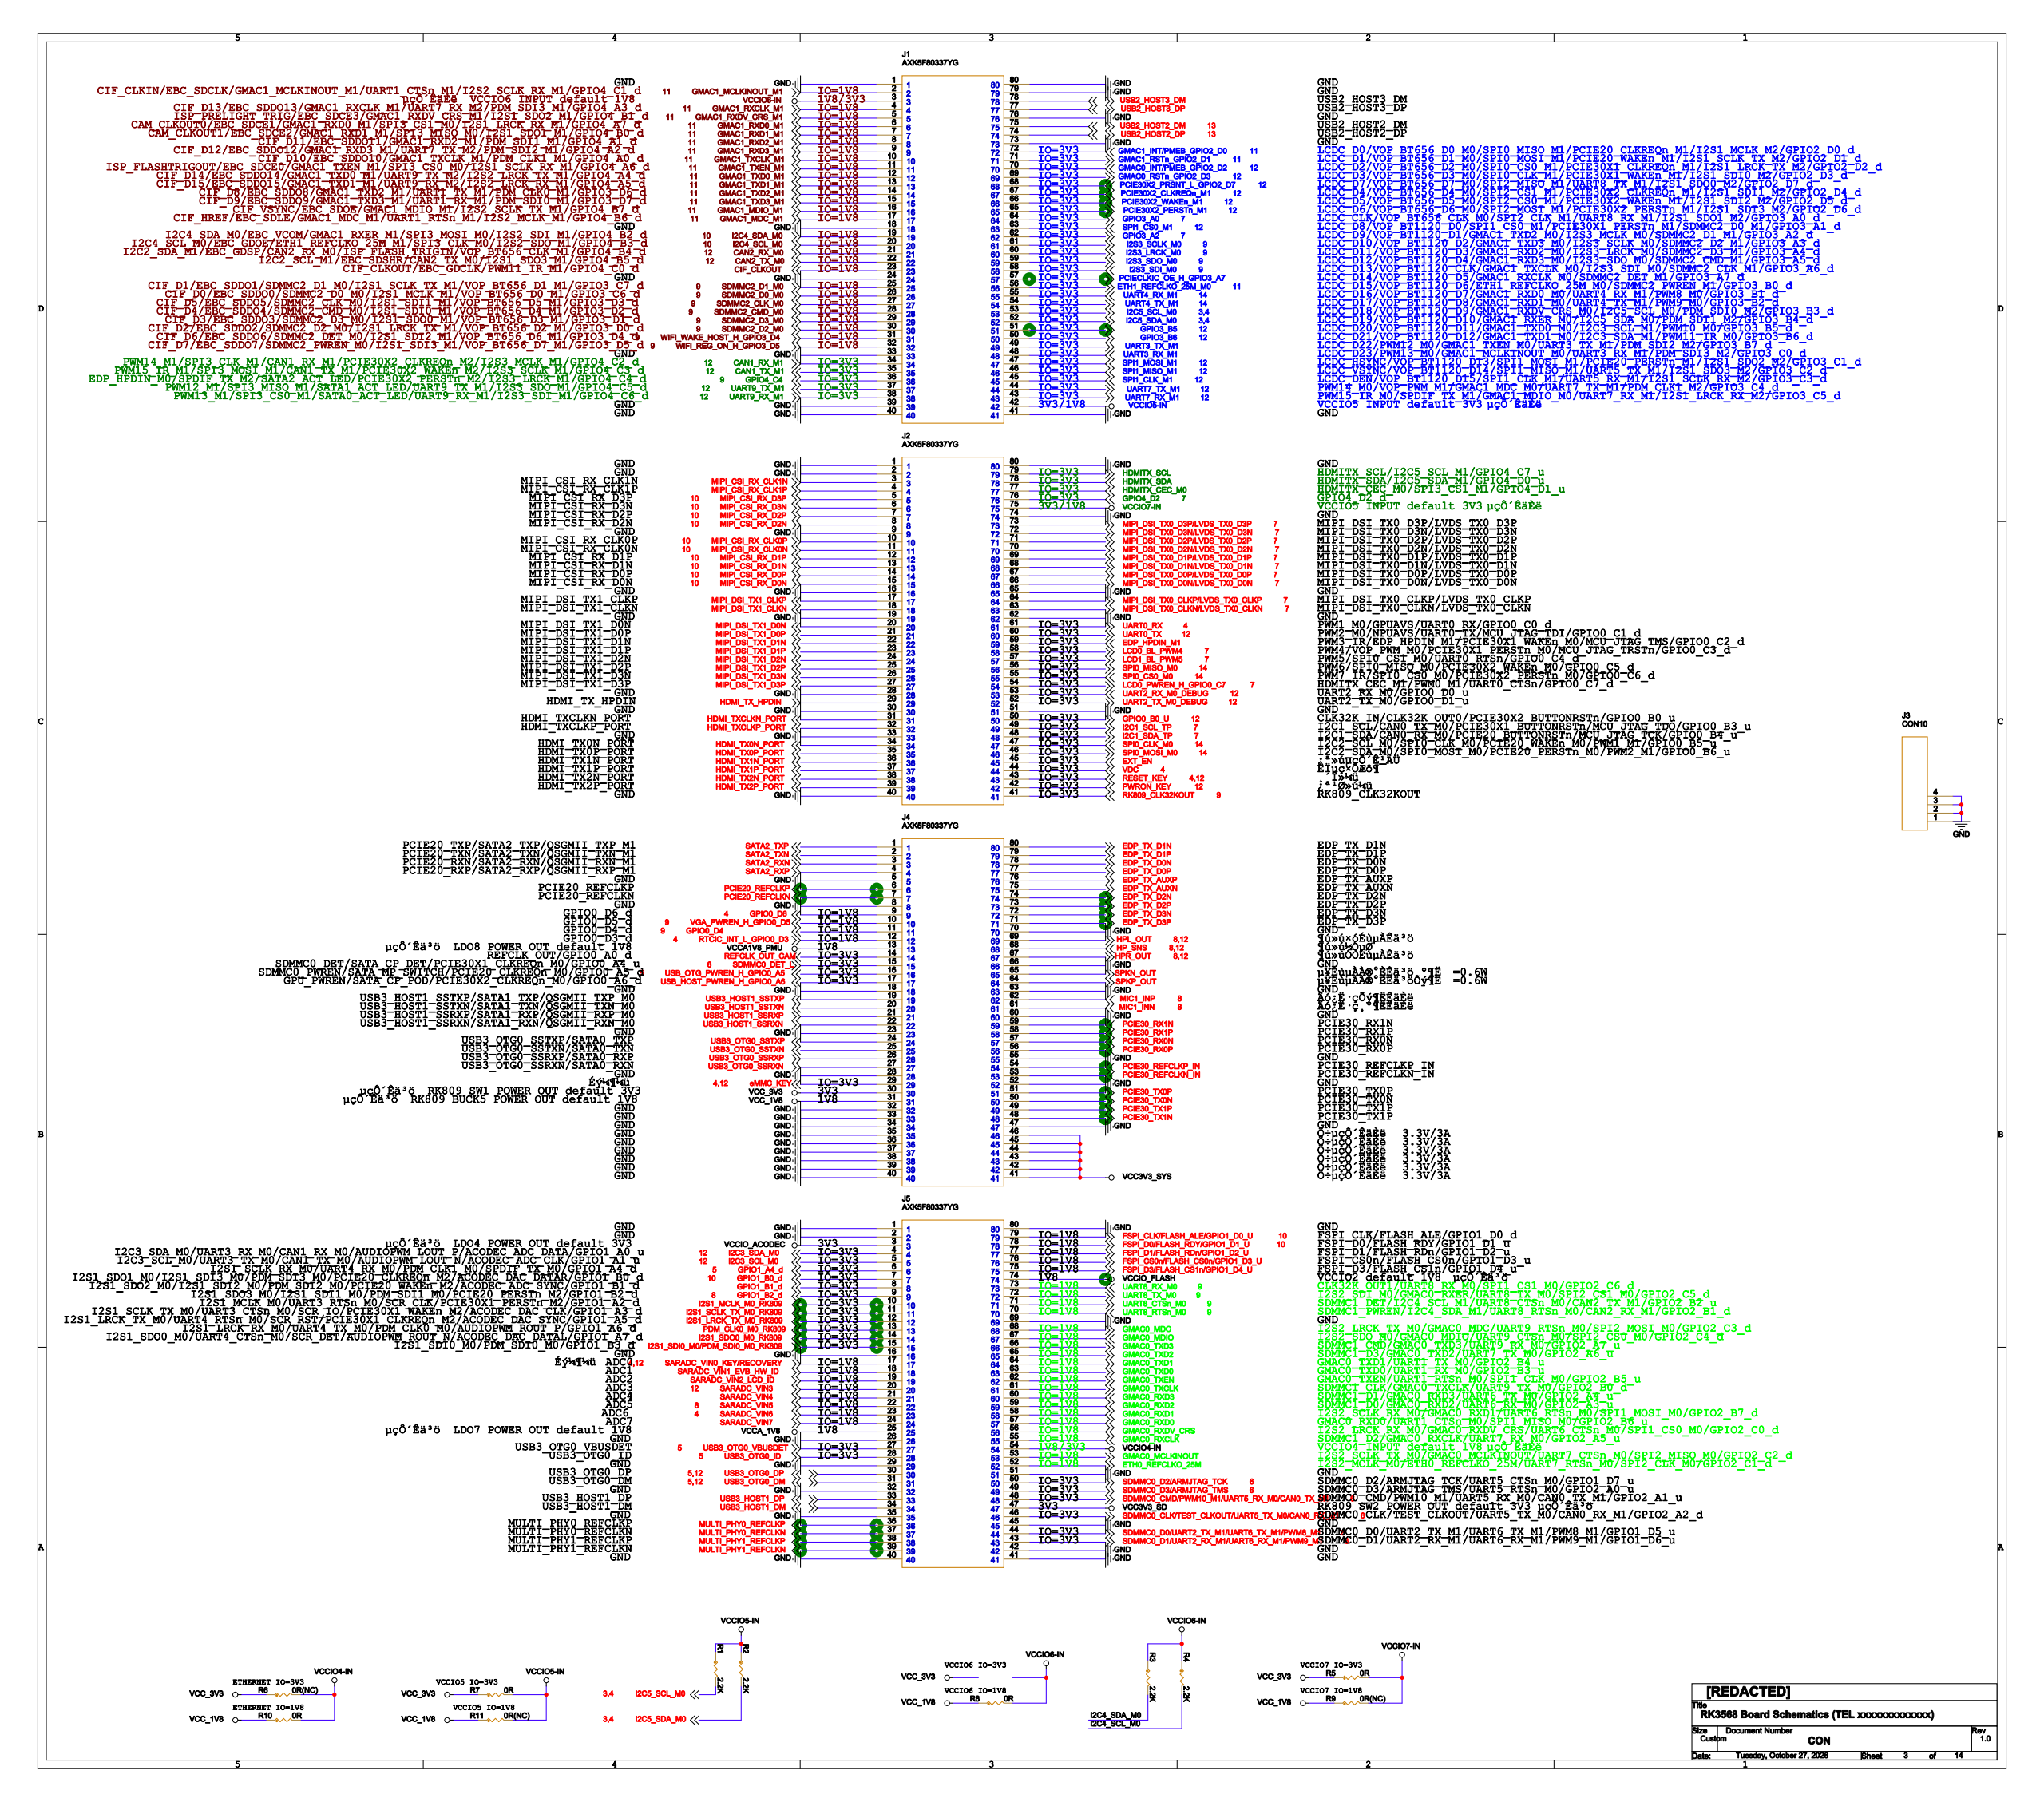Circuit board | Cadence Allegro | 669 parts | 581 nets | one sheet of the schematic
Parts on this sheet (reference | value | footprint):
J1 | AXK5F80337YG | AXK5F80337YG
J2 | AXK5F80337YG | AXK5F80337YG
J3 | CON10 | DIP-CORE-A40I
J4 | AXK5F80337YG | AXK5F80337YG
J5 | AXK5F80337YG | AXK5F80337YG
R1 | 2.2K | R0402
R2 | 2.2K | R0402
R3 | 2.2K | R0402
R4 | 2.2K | R0402
R5 | 0R | R0402
R6 | 0R(NC) | R0402
R7 | 0R | R0402
R8 | 0R | R0402
R9 | 0R(NC) | R0402
R10 | 0R | R0402
R11 | 0R(NC) | R0402
Nets of these parts (net: part-pin ...):
GND: J3-1 J3-2 J3-3 J3-4 J1-1 J1-18 J1-24 J1-33 J1-39 J1-40 J1-41 J1-73 J1-76 J1-79 J1-80 J2-1 J2-2 J2-9 J2-16 J2-19 J2-28 J2-30 J2-33 J2-40 J2-51 J2-62 J2-65 J2-74 J2-80 J4-5 J4-8 J4-18 J4-23 J4-28 J4-32 J4-33 J4-34 J4-35 J4-36 J4-37 J4-38 J4-39 J4-40 J4-47 J4-52 J4-55 J4-60 J4-63 J4-66 J4-70 J5-1 J5-2 J5-16 J5-26 J5-29 J5-32 J5-35 J5-40 J5-41 J5-42 J5-45 J5-51 J5-69 J5-80
SARADC_VIN6: J5-23
VCC3V3_SYS: J4-41 J4-42 J4-43 J4-44 J4-45 J4-46
SARADC_VIN5: J5-22
VCCIO6-IN: R3-1 R4-1 R8-2 J1-3
HPR_OUT: J4-67
HPL_OUT: J4-69
MIC1_INP: J4-62
MIC1_INN: J4-61
RESET_KEY: J2-43
PWRON_KEY: J2-42
USB3_OTG0_VBUSDET: J5-27
VCC3V3_SD: J5-47
SPI1_CLK_M1: J1-45
UART3_RX_M1: J1-48
UART3_TX_M1: J1-49
GPIO3_B6: J1-50
GPIO3_B5: J1-51
SPI1_CS0_M1: J1-63
PCIE30X2_PRSNT_L_GPIO2_D7: J1-68
UART0_RX: J2-61
GPIO4_D2: J2-76
UART7_RX_M1: J1-43
UART7_TX_M1: J1-44
SARADC_VIN0_KEY/RECOVERY: J5-17
USB3_OTG0_DP: J5-30
USB3_OTG0_DM: J5-31
SDMMC0_D2/ARMJTAG_TCK: J5-50
SDMMC0_D3/ARMJTAG_TMS: J5-49
SDMMC0_DET_L: J4-15
USB2_HOST2_DP: J1-74
USB2_HOST2_DM: J1-75
MIPI_DSI_TX0_D2N/LVDS_TX0_D2N: J2-70
MIPI_DSI_TX0_D2P/LVDS_TX0_D2P: J2-71
MIPI_DSI_TX0_CLKN/LVDS_TX0_CLKN: J2-63
MIPI_DSI_TX0_CLKP/LVDS_TX0_CLKP: J2-64
MIPI_DSI_TX0_D3N/LVDS_TX0_D3N: J2-72
MIPI_DSI_TX0_D3P/LVDS_TX0_D3P: J2-73
MIPI_DSI_TX0_D0N/LVDS_TX0_D0N: J2-66
MIPI_DSI_TX0_D0P/LVDS_TX0_D0P: J2-67
MIPI_DSI_TX0_D1N/LVDS_TX0_D1N: J2-68
MIPI_DSI_TX0_D1P/LVDS_TX0_D1P: J2-69
VCC_3V3: R5-1 R6-1 R7-1 J4-30
UART2_RX_M0_DEBUG: J2-53
VCC_1V8: R8-1 R9-1 R10-1 R11-1 J4-31
VCCIO5-IN: R1-1 R2-1 R7-2 R11-2 J1-42
VCCIO4-IN: R6-2 R10-2 J5-54
VCCIO7-IN: R5-2 R9-2 J2-75
RK809_CLK32KOUT: J2-41
I2C4_SCL_M0: R4-2 J1-20
I2C4_SDA_M0: R3-2 J1-19
FSPI_D0/FLASH_RDY/GPIO1_D1_U: J5-78
I2C1_SDA_TP: J2-48
I2C1_SCL_TP: J2-49
GPIO3_A2: J1-62
GPIO3_A0: J1-64
HP_SNS: J4-68
CAN2_RX_M0: J1-21
CAN2_TX_M0: J1-22
GMAC1_INT/PMEB_GPIO2_D0: J1-72
VCCA1V8_PMU: J4-13
RTCIC_INT_L_GPIO0_D3: J4-12
SARADC_VIN3: J5-20
VCCA_1V8: J5-25
GMAC0_INT/PMEB_GPIO2_D2: J1-70
FSPI_CLK/FLASH_ALE/GPIO1_D0_U: J5-79
GMAC1_RXD0_M1: J1-6
GMAC1_RXD1_M1: J1-7
GMAC1_RXD2_M1: J1-8
GMAC1_MCLKINOUT_M1: J1-2
ETH1_REFCLKO_25M_M0: J1-56
UART2_TX_M0_DEBUG: J2-52
USB3_OTG0_ID: J5-28
VCCIO_ACODEC: J5-3
LCD0_PWREN_H_GPIO0_C7: J2-54
UART0_TX: J2-60
UART9_TX_M1: J1-37
VDC: J2-44
GPIO0_D6: J4-9
GMAC1_RXD3_M1: J1-9
GMAC1_RXCLK_M1: J1-4
GMAC1_RXDV_CRS_M1: J1-5
GMAC1_MDIO_M1: J1-16
UART9_RX_M1: J1-38
CAN1_RX_M1: J1-34
I2C5_SCL_M0: R1-2 J1-53
I2C5_SDA_M0: R2-2 J1-52
EXT_EN: J2-45
EDP_HPDIN_M1: J2-59
LCD0_BL_PWM4: J2-58
LCD1_BL_PWM5: J2-57
GPIO0_D4: J4-11
GPIO4_C4: J1-36
VGA_PWREN_H_GPIO0_D5: J4-10
SDMMC2_D0_M0: J1-26
SDMMC2_D1_M0: J1-25
SDMMC2_D2_M0: J1-30
SDMMC2_D3_M0: J1-29
SDMMC2_CLK_M0: J1-27
SDMMC2_CMD_M0: J1-28
UART8_TX_M0: J5-72
UART8_RX_M0: J5-73
WIFI_WAKE_HOST_H_GPIO3_D4: J1-31
WIFI_REG_ON_H_GPIO3_D5: J1-32
GMAC1_MDC_M1: J1-17
GMAC1_TXCLK_M1: J1-10
GMAC1_TXEN_M1: J1-11
GMAC1_TXD0_M1: J1-12
GMAC1_TXD1_M1: J1-13
GMAC1_TXD2_M1: J1-14
GMAC1_TXD3_M1: J1-15
GPIO0_B0_U: J2-50
SPI1_MOSI_M1: J1-47
SPI1_MISO_M1: J1-46
I2C3_SCL_M0: J5-5
I2C3_SDA_M0: J5-4
CAN1_TX_M1: J1-35
USB_OTG_PWREN_H_GPIO0_A5: J4-16
UART4_RX_M1: J1-55
UART4_TX_M1: J1-54
I2S3_SDI_M0: J1-58
I2S3_SCLK_M0: J1-61
I2S3_SDO_M0: J1-59
I2S3_LRCK_M0: J1-60
MIPI_CSI_RX_CLK0N: J2-11
MIPI_CSI_RX_CLK0P: J2-10
MIPI_CSI_RX_D0N: J2-15
MIPI_CSI_RX_D1N: J2-13
MIPI_CSI_RX_D2N: J2-8
MIPI_CSI_RX_D3N: J2-6
MIPI_CSI_RX_D0P: J2-14
MIPI_CSI_RX_D1P: J2-12
MIPI_CSI_RX_D2P: J2-7
MIPI_CSI_RX_D3P: J2-5
CIF_CLKOUT: J1-23
PCIECLKIC_OE_H_GPIO3_A7: J1-57
USB2_HOST3_DP: J1-77
USB2_HOST3_DM: J1-78
MIPI_DSI_TX1_CLKP: J2-17
MIPI_DSI_TX1_CLKN: J2-18
MIPI_DSI_TX1_D0N: J2-20
MIPI_DSI_TX1_D0P: J2-21
MIPI_DSI_TX1_D1N: J2-22
MIPI_DSI_TX1_D1P: J2-23
MIPI_DSI_TX1_D2N: J2-24
MIPI_DSI_TX1_D2P: J2-25
MIPI_DSI_TX1_D3N: J2-26
MIPI_DSI_TX1_D3P: J2-27
HDMI_TX_HPDIN: J2-29
MIPI_CSI_RX_CLK1N: J2-3
HDMI_TXCLKN_PORT: J2-31
HDMI_TXCLKP_PORT: J2-32
HDMI_TX0N_PORT: J2-34
HDMI_TX0P_PORT: J2-35
HDMI_TX1N_PORT: J2-36
HDMI_TX1P_PORT: J2-37
HDMI_TX2N_PORT: J2-38
HDMI_TX2P_PORT: J2-39
MIPI_CSI_RX_CLK1P: J2-4
HDMITX_CEC_M0: J2-77
HDMITX_SDA: J2-78
HDMITX_SCL: J2-79
SATA2_TXP: J4-1
REFCLK_OUT_CAM: J4-14
USB_HOST_PWREN_H_GPIO0_A6: J4-17
USB3_HOST1_SSTXP: J4-19
SATA2_TXN: J4-2
USB3_HOST1_SSTXN: J4-20
USB3_HOST1_SSRXP: J4-21
USB3_HOST1_SSRXN: J4-22
USB3_OTG0_SSTXP: J4-24
USB3_OTG0_SSTXN: J4-25
USB3_OTG0_SSRXP: J4-26
USB3_OTG0_SSRXN: J4-27
SATA2_RXN: J4-3
SATA2_RXP: J4-4
PCIE30_TX1N: J4-48
PCIE30_TX1P: J4-49
PCIE30_TX0N: J4-50
PCIE30_TX0P: J4-51
PCIE30_REFCLKN_IN: J4-53
PCIE30_REFCLKP_IN: J4-54
PCIE30_RX0P: J4-56
PCIE30_RX0N: J4-57
PCIE30_RX1P: J4-58
PCIE30_RX1N: J4-59
PCIE20_REFCLKP: J4-6
SPKP_OUT: J4-64
SPKN_OUT: J4-65
PCIE20_REFCLKN: J4-7
EDP_TX_D3P: J4-71
EDP_TX_D3N: J4-72
EDP_TX_D2P: J4-73
EDP_TX_D2N: J4-74
EDP_TX_AUXN: J4-75
EDP_TX_AUXP: J4-76
EDP_TX_D0P: J4-77
EDP_TX_D0N: J4-78
EDP_TX_D1P: J4-79
EDP_TX_D1N: J4-80
I2S1_MCLK_M0_RK809: J5-10
I2S1_SCLK_TX_M0_RK809: J5-11
I2S1_LRCK_TX_M0_RK809: J5-12
PDM_CLK0_M0_RK809: J5-13
I2S1_SDO0_M0_RK809: J5-14
I2S1_SDI0_M0/PDM_SDI0_M0_RK809: J5-15
SARADC_VIN1_EVB_HW_ID: J5-18
SARADC_VIN2_LCD_ID: J5-19
SARADC_VIN4: J5-21
SARADC_VIN7: J5-24
USB3_HOST1_DP: J5-33
USB3_HOST1_DM: J5-34
MULTI_PHY0_REFCLKP: J5-36
MULTI_PHY0_REFCLKN: J5-37
MULTI_PHY1_REFCLKP: J5-38
MULTI_PHY1_REFCLKN: J5-39
ETH0_REFCLKO_25M: J5-52
GMAC0_MCLKINOUT: J5-53
GMAC0_RXCLK: J5-55
GMAC0_RXDV_CRS: J5-56
GMAC0_RXD0: J5-57
GMAC0_RXD1: J5-58
GMAC0_RXD2: J5-59
GMAC0_RXD3: J5-60
GMAC0_TXCLK: J5-61
GMAC0_TXEN: J5-62
GMAC0_TXD0: J5-63
GMAC0_TXD1: J5-64
GMAC0_TXD2: J5-65
GMAC0_TXD3: J5-66
GMAC0_MDIO: J5-67
GMAC0_MDC: J5-68
VCCIO_FLASH: J5-74